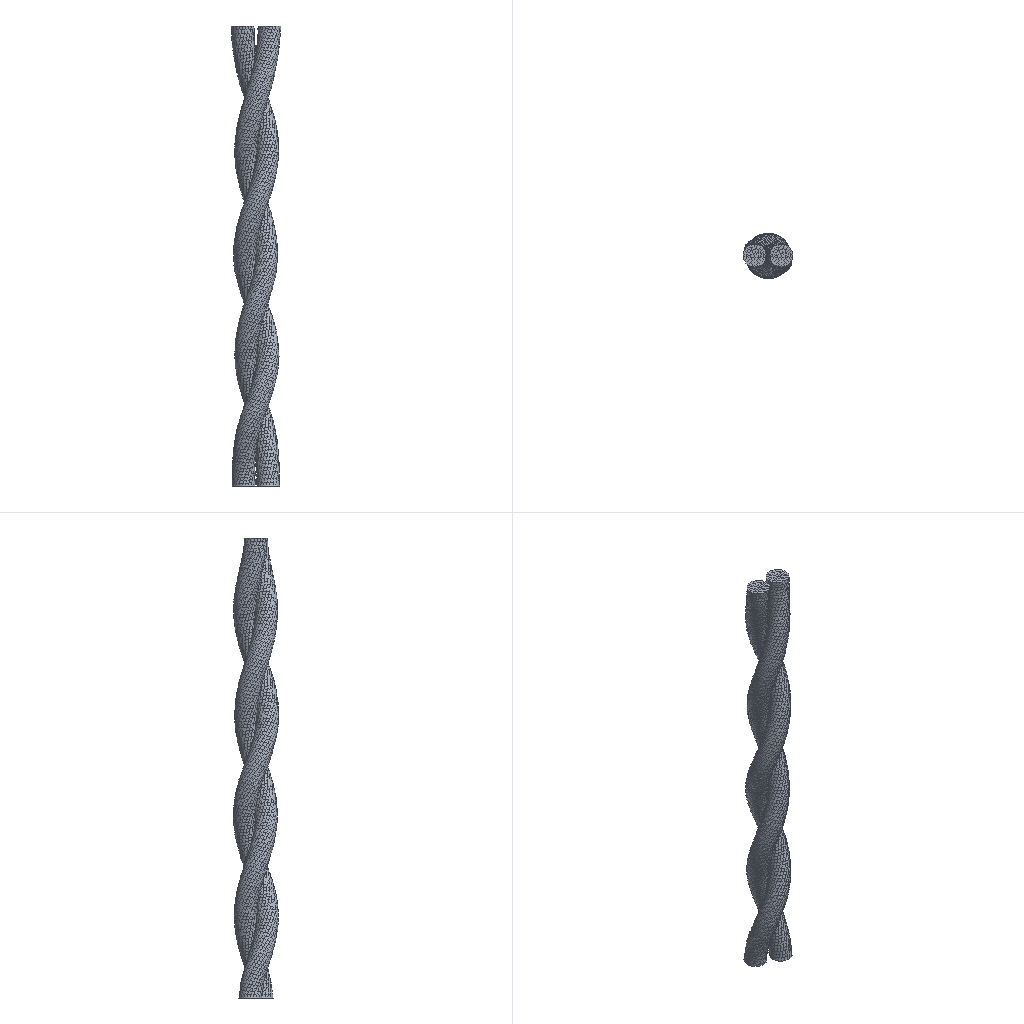Simulation study | abaqus
Set-up summary:
category,name,step,type,value,unit,region
solver,abaqus
solver,version,,,Abaqus/Explicit 2020
units,not stated in the deck,,not stated
analysis,deck,,transient,transient
load_step,Step-2,Step-2,transient,nlgeom=True
contact,interactions,,,general=1 pairs=0 ties=0
load_step,requested,,,1
mesh,nodes,,,19312
mesh,elements,,,15792
element_type,C3D8R,,solid,15792
load,load commands in deck,,count,1
bc,support commands in deck,,count,7
material,MATERIAL-1,,in results
check,setup vs results,,match,"per instance, exact: element labels, types and connectivity; labels of the nodes the elements use; coordinates of those nodes at SINGLE_PRECISION in 2 of 2 instance(s)"
Abaqus input file, long lists of numbers shortened:
*Heading
** Job name: Job-7 Model name: new-2
** Generated by: Abaqus/CAE 2020
*Preprint, echo=NO, model=NO, history=NO, contact=NO
**
** PARTS
**
*Part, name=PART-2-1
*Node
      1, 0.00727, -0.01485,           0.
      2, 0.02272, -0.008,           0.
** (9654 more lines like these left out)
*Element, type=C3D8R
2007, 2498, 2477, 2483, 2509, 2430, 2409, 2415, 2441
1994, 2474, 2491, 2509, 2483, 2406, 2423, 2441, 2415
** (7894 more lines like these left out)
*Nset, nset=SET-1, generate
    1,  9656,     1
*Elset, elset=SET-1, generate
    1,  7896,     1
*Elset, elset=Set-2, generate
    1,  7896,     1
*Orientation, name=Ori-1
1., 0., 0., 0., 1., 0.
1, 0.
** Section: Section-1
*Solid Section, elset=Set-2, orientation=Ori-1, material=Material-1
,
*End Part
**
*Part, name=PART-2-1-LIN-2-1
*Node
      1, 0.07062, -0.04462,           0.
      2, 0.08607, -0.03777,           0.
** (9654 more lines like these left out)
*Element, type=C3D8R
1914, 2412, 2392, 2402, 2421, 2344, 2324, 2334, 2353
1921, 2391, 2405, 2421, 2402, 2323, 2337, 2353, 2334
** (7894 more lines like these left out)
*Nset, nset=SET-1, generate
    1,  9656,     1
*Elset, elset=SET-1, generate
    1,  7896,     1
*Elset, elset=Set-2, generate
    1,  7896,     1
*Orientation, name=Ori-1
1., 0., 0., 0., 1., 0.
1, 0.
** Section: Section-1
*Solid Section, elset=Set-2, orientation=Ori-1, material=Material-1
,
*End Part
**
**
** ASSEMBLY
**
*Assembly, name=Assembly
**
*Instance, name=PART-2-1-2, part=PART-2-1
*End Instance
**
*Instance, name=PART-2-1-LIN-2-1-2, part=PART-2-1-LIN-2-1
*End Instance
**
*Node
      1, 0.035, 2.88709998e-08,           0.
*Nset, nset=Set-17
 1,
*Nset, nset=Set-18, instance=PART-2-1-2, generate
 9589,  9656,     1
*Nset, nset=Set-18, instance=PART-2-1-LIN-2-1-2, generate
 9589,  9656,     1
*Nset, nset=Set-19, instance=PART-2-1-2, generate
    1,  9656,     1
*Nset, nset=Set-19, instance=PART-2-1-LIN-2-1-2, generate
    1,  9656,     1
*Nset, nset=m_Set-16
 1,
*Elset, elset=_s_Surf-5_S2, internal, instance=PART-2-1-2, generate
  1,  56,   1
*Elset, elset=_s_Surf-5_S2, internal, instance=PART-2-1-LIN-2-1-2, generate
  1,  56,   1
*Surface, type=ELEMENT, name=s_Surf-5
_s_Surf-5_S2, S2
** Constraint: Constraint-2
*Coupling, constraint name=Constraint-2, ref node=m_Set-16, surface=s_Surf-5
*Kinematic
*End Assembly
*Amplitude, name=Amp-1
             0.,              0.,            0.01,              1.
**
** MATERIALS
**
*Material, name=Material-1
*Density
 1.5e-09,
*Elastic
1600., 0.35
*Expansion, type=ORTHO
 0.008,  0.008, -0.001
**
** INTERACTION PROPERTIES
**
*Surface Interaction, name=IntProp-1
*Friction
 0.05,
*Surface Behavior, pressure-overclosure=HARD
**
** PREDEFINED FIELDS
**
** Name: Predefined Field-1   Type: Temperature
*Initial Conditions, type=TEMPERATURE
Set-19, 0.
** ----------------------------------------------------------------
**
** STEP: Step-2
**
*Step, name=Step-2, nlgeom=YES
*Dynamic, Explicit
, 0.0035
*Bulk Viscosity
0.06, 1.2
** Mass Scaling: Semi-Automatic
**               Whole Model
*Fixed Mass Scaling, factor=50.
**
** BOUNDARY CONDITIONS
**
** Name: BC-2 Type: 位移/转角
*Boundary, amplitude=Amp-1
Set-17, 1, 1
Set-17, 2, 2
Set-17, 4, 4
Set-17, 5, 5
** Name: BC-3 Type: 位移/转角
*Boundary
Set-18, 1, 1
Set-18, 2, 2
Set-18, 3, 3
**
** PREDEFINED FIELDS
**
** Name: Predefined Field-1   Type: Temperature
*Temperature, amplitude=Amp-1
Set-19, 250.
**
** INTERACTIONS
**
** Interaction: Int-2
*Contact, op=NEW
*Contact Inclusions, ALL EXTERIOR
*Contact Property Assignment
 ,  , IntProp-1
**
** OUTPUT REQUESTS
**
*Restart, write, number interval=1, time marks=NO
**
** FIELD OUTPUT: F-Output-2
**
*Output, field, number interval=30
*Node Output
A, CF, RF, RT, U, V
*Element Output, directions=YES
E, LE, MISES, MISESMAX, MISESONLY, NE, PEEQ, PEEQVAVG, PRESSONLY, S, SEQUT, SF, SSAVG, SVAVG, YIELDPOT
*Contact Output
CDISP, CFORCE, CSTRESS, FSLIP, FSLIPR, PPRESS
*Output, history, frequency=0
*End Step
Results summary:
result,step,Step-2,completed,increments=166153 time=0.0035/0.0035
result,analysis,,,transient
result,last_loadstep,,,1
result,analysis steps,,count,1
result,primary field,,,U
result,reaction total,,FX,-0.002115,model units
result,reaction total,,FY,-0.01222,model units
result,reaction total,,FZ,-0.000105,model units